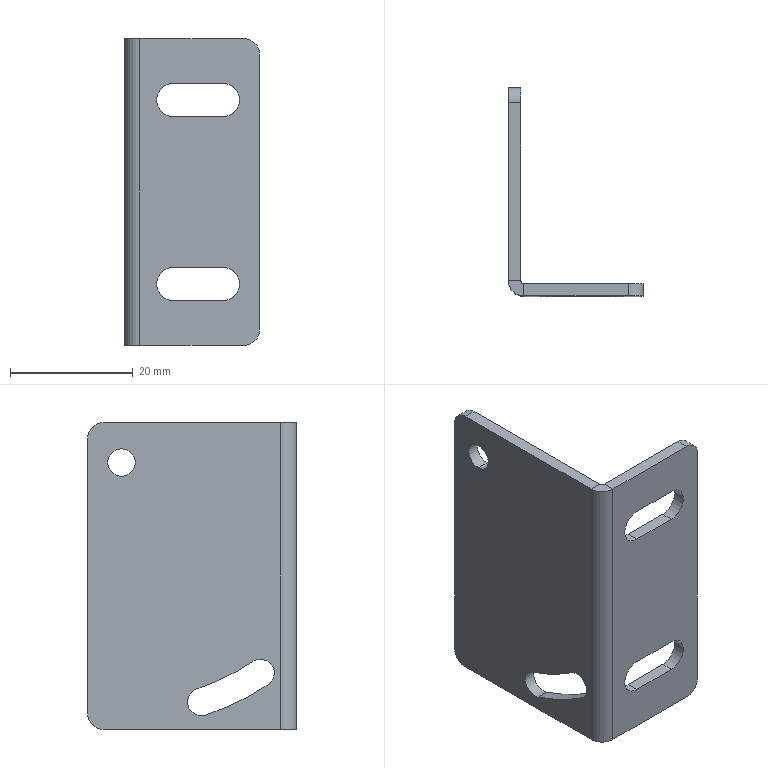Part | STEP file | KF-2212-060-004 | 1 solid | 33 faces | box 22 x 34 x 50 mm | volume 4893 mm3 | cylinder 17 | plane 16 | commonest cylinder face diameters 4.5 x5 5 x5 5.5 x4 1 x1 77.792 x1 86.792 x1
STEP:
#1=CARTESIAN_POINT('',(0.,26.5,45.75));
#2=VERTEX_POINT('',#1);
#3=CARTESIAN_POINT('',(0.,26.5,41.25));
#4=VERTEX_POINT('',#3);
#5=CARTESIAN_POINT('',(0.,26.5,43.5));
#6=DIRECTION('',(1.,0.,0.));
#7=DIRECTION('',(0.,0.,-1.));
#8=AXIS2_PLACEMENT_3D('',#5,#6,#7);
#9=CIRCLE('',#8,2.25);
#10=EDGE_CURVE('',#2,#4,#9,.T.);
#11=ORIENTED_EDGE('',*,*,#10,.T.);
#12=CARTESIAN_POINT('',(-2.,26.5,41.25));
#13=VERTEX_POINT('',#12);
#14=CARTESIAN_POINT('',(8.,26.5,41.25));
#15=DIRECTION('',(-1.,0.,0.));
#16=VECTOR('',#15,1000.);
#17=LINE('',#14,#16);
#18=EDGE_CURVE('',#4,#13,#17,.T.);
#19=ORIENTED_EDGE('',*,*,#18,.T.);
#20=CARTESIAN_POINT('',(-2.,26.5,45.75));
#21=VERTEX_POINT('',#20);
#22=CARTESIAN_POINT('',(-2.,26.5,43.5));
#23=DIRECTION('',(-1.,0.,0.));
#24=DIRECTION('',(0.,0.,1.));
#25=AXIS2_PLACEMENT_3D('',#22,#23,#24);
#26=CIRCLE('',#25,2.25);
#27=EDGE_CURVE('',#13,#21,#26,.T.);
#28=ORIENTED_EDGE('',*,*,#27,.T.);
#29=CARTESIAN_POINT('',(8.,26.5,45.75));
#30=DIRECTION('',(-1.,0.,0.));
#31=VECTOR('',#30,1000.);
#32=LINE('',#29,#31);
#33=EDGE_CURVE('',#2,#21,#32,.T.);
#34=ORIENTED_EDGE('',*,*,#33,.F.);
#35=EDGE_LOOP('',(#11,#19,#28,#34));
#36=FACE_OUTER_BOUND('',#35,.T.);
#37=CARTESIAN_POINT('',(8.,26.5,43.5));
#38=DIRECTION('',(-1.,0.,0.));
#39=DIRECTION('',(0.,0.,1.));
#40=AXIS2_PLACEMENT_3D('',#37,#38,#39);
#41=CYLINDRICAL_SURFACE('',#40,2.25);
#42=ADVANCED_FACE('',(#36),#41,.F.);
#43=CARTESIAN_POINT('',(0.,5.064,11.044));
#44=VERTEX_POINT('',#43);
#45=CARTESIAN_POINT('',(0.,3.825,11.416));
#46=VERTEX_POINT('',#45);
#47=CARTESIAN_POINT('',(0.,3.825,9.166));
#48=DIRECTION('',(1.,0.,0.));
#49=DIRECTION('',(0.,0.,-1.));
#50=AXIS2_PLACEMENT_3D('',#47,#48,#49);
#51=CIRCLE('',#50,2.25);
#52=EDGE_CURVE('',#44,#46,#51,.T.);
#53=ORIENTED_EDGE('',*,*,#52,.T.);
#54=CARTESIAN_POINT('',(-2.,3.825,11.416));
#55=VERTEX_POINT('',#54);
#56=CARTESIAN_POINT('',(8.,3.825,11.416));
#57=DIRECTION('',(-1.,0.,0.));
#58=VECTOR('',#57,1000.);
#59=LINE('',#56,#58);
#60=EDGE_CURVE('',#46,#55,#59,.T.);
#61=ORIENTED_EDGE('',*,*,#60,.T.);
#62=CARTESIAN_POINT('',(-2.,5.064,11.044));
#63=VERTEX_POINT('',#62);
#64=CARTESIAN_POINT('',(-2.,3.825,9.166));
#65=DIRECTION('',(-1.,0.,0.));
#66=DIRECTION('',(0.,0.,1.));
#67=AXIS2_PLACEMENT_3D('',#64,#65,#66);
#68=CIRCLE('',#67,2.25);
#69=EDGE_CURVE('',#55,#63,#68,.T.);
#70=ORIENTED_EDGE('',*,*,#69,.T.);
#71=CARTESIAN_POINT('',(8.,5.064,11.044));
#72=DIRECTION('',(-1.,0.,0.));
#73=VECTOR('',#72,1000.);
#74=LINE('',#71,#73);
#75=EDGE_CURVE('',#44,#63,#74,.T.);
#76=ORIENTED_EDGE('',*,*,#75,.F.);
#77=EDGE_LOOP('',(#53,#61,#70,#76));
#78=FACE_OUTER_BOUND('',#77,.T.);
#79=CARTESIAN_POINT('',(8.,3.825,9.166));
#80=DIRECTION('',(-1.,0.,0.));
#81=DIRECTION('',(0.,0.,1.));
#82=AXIS2_PLACEMENT_3D('',#79,#80,#81);
#83=CYLINDRICAL_SURFACE('',#82,2.25);
#84=ADVANCED_FACE('',(#78),#83,.F.);
#85=CARTESIAN_POINT('',(0.5,0.,50.));
#86=VERTEX_POINT('',#85);
#87=CARTESIAN_POINT('',(0.5,-2.,50.));
#88=VERTEX_POINT('',#87);
#89=CARTESIAN_POINT('',(0.5,0.,50.));
#90=DIRECTION('',(0.,-1.,0.));
#91=VECTOR('',#90,1000.);
#92=LINE('',#89,#91);
#93=EDGE_CURVE('',#86,#88,#92,.T.);
#94=ORIENTED_EDGE('',*,*,#93,.F.);
#95=CARTESIAN_POINT('',(0.,0.5,50.));
#96=VERTEX_POINT('',#95);
#97=CARTESIAN_POINT('',(0.5,0.5,50.));
#98=DIRECTION('',(0.,0.,1.));
#99=DIRECTION('',(-1.,0.,0.));
#100=AXIS2_PLACEMENT_3D('',#97,#98,#99);
#101=CIRCLE('',#100,0.5);
#102=EDGE_CURVE('',#96,#86,#101,.T.);
#103=ORIENTED_EDGE('',*,*,#102,.F.);
#104=CARTESIAN_POINT('',(-2.,0.5,50.));
#105=VERTEX_POINT('',#104);
#106=CARTESIAN_POINT('',(-2.,0.5,50.));
#107=DIRECTION('',(1.,0.,0.));
#108=VECTOR('',#107,1000.);
#109=LINE('',#106,#108);
#110=EDGE_CURVE('',#105,#96,#109,.T.);
#111=ORIENTED_EDGE('',*,*,#110,.F.);
#112=CARTESIAN_POINT('',(0.5,0.5,50.));
#113=DIRECTION('',(0.,0.,1.));
#114=DIRECTION('',(1.,0.,0.));
#115=AXIS2_PLACEMENT_3D('',#112,#113,#114);
#116=CIRCLE('',#115,2.5);
#117=EDGE_CURVE('',#105,#88,#116,.T.);
#118=ORIENTED_EDGE('',*,*,#117,.T.);
#119=EDGE_LOOP('',(#94,#103,#111,#118));
#120=FACE_OUTER_BOUND('',#119,.T.);
#121=CARTESIAN_POINT('',(0.5,0.,50.));
#122=DIRECTION('',(0.,0.,1.));
#123=DIRECTION('',(1.,0.,0.));
#124=AXIS2_PLACEMENT_3D('',#121,#122,#123);
#125=PLANE('',#124);
#126=ADVANCED_FACE('',(#120),#125,.T.);
#127=CARTESIAN_POINT('',(17.5,-2.,50.));
#128=VERTEX_POINT('',#127);
#129=CARTESIAN_POINT('',(0.,-2.,50.));
#130=DIRECTION('',(1.,0.,0.));
#131=VECTOR('',#130,1000.);
#132=LINE('',#129,#131);
#133=EDGE_CURVE('',#88,#128,#132,.T.);
#134=ORIENTED_EDGE('',*,*,#133,.T.);
#135=CARTESIAN_POINT('',(17.5,0.,50.));
#136=VERTEX_POINT('',#135);
#137=CARTESIAN_POINT('',(17.5,0.5,50.));
#138=DIRECTION('',(0.,1.,0.));
#139=VECTOR('',#138,1000.);
#140=LINE('',#137,#139);
#141=EDGE_CURVE('',#128,#136,#140,.T.);
#142=ORIENTED_EDGE('',*,*,#141,.T.);
#143=CARTESIAN_POINT('',(0.,0.,50.));
#144=DIRECTION('',(1.,0.,0.));
#145=VECTOR('',#144,1000.);
#146=LINE('',#143,#145);
#147=EDGE_CURVE('',#86,#136,#146,.T.);
#148=ORIENTED_EDGE('',*,*,#147,.F.);
#149=ORIENTED_EDGE('',*,*,#93,.T.);
#150=EDGE_LOOP('',(#134,#142,#148,#149));
#151=FACE_OUTER_BOUND('',#150,.T.);
#152=CARTESIAN_POINT('',(-2.,0.5,50.));
#153=DIRECTION('',(0.,0.,1.));
#154=DIRECTION('',(1.,0.,0.));
#155=AXIS2_PLACEMENT_3D('',#152,#153,#154);
#156=PLANE('',#155);
#157=ADVANCED_FACE('',(#151),#156,.T.);
#158=CARTESIAN_POINT('',(0.,0.5,0.));
#159=VERTEX_POINT('',#158);
#160=CARTESIAN_POINT('',(-2.,0.5,0.));
#161=VERTEX_POINT('',#160);
#162=CARTESIAN_POINT('',(0.,0.5,0.));
#163=DIRECTION('',(-1.,0.,0.));
#164=VECTOR('',#163,1000.);
#165=LINE('',#162,#164);
#166=EDGE_CURVE('',#159,#161,#165,.T.);
#167=ORIENTED_EDGE('',*,*,#166,.F.);
#168=CARTESIAN_POINT('',(0.5,0.,0.));
#169=VERTEX_POINT('',#168);
#170=CARTESIAN_POINT('',(0.5,0.5,0.));
#171=DIRECTION('',(0.,0.,1.));
#172=DIRECTION('',(-1.,0.,0.));
#173=AXIS2_PLACEMENT_3D('',#170,#171,#172);
#174=CIRCLE('',#173,0.5);
#175=EDGE_CURVE('',#159,#169,#174,.T.);
#176=ORIENTED_EDGE('',*,*,#175,.T.);
#177=CARTESIAN_POINT('',(0.5,-2.,0.));
#178=VERTEX_POINT('',#177);
#179=CARTESIAN_POINT('',(0.5,-2.,0.));
#180=DIRECTION('',(0.,1.,0.));
#181=VECTOR('',#180,1000.);
#182=LINE('',#179,#181);
#183=EDGE_CURVE('',#178,#169,#182,.T.);
#184=ORIENTED_EDGE('',*,*,#183,.F.);
#185=CARTESIAN_POINT('',(0.5,0.5,0.));
#186=DIRECTION('',(0.,0.,1.));
#187=DIRECTION('',(1.,0.,0.));
#188=AXIS2_PLACEMENT_3D('',#185,#186,#187);
#189=CIRCLE('',#188,2.5);
#190=EDGE_CURVE('',#161,#178,#189,.T.);
#191=ORIENTED_EDGE('',*,*,#190,.F.);
#192=EDGE_LOOP('',(#167,#176,#184,#191));
#193=FACE_OUTER_BOUND('',#192,.T.);
#194=CARTESIAN_POINT('',(0.,0.5,0.));
#195=DIRECTION('',(0.,0.,-1.));
#196=DIRECTION('',(-1.,0.,0.));
#197=AXIS2_PLACEMENT_3D('',#194,#195,#196);
#198=PLANE('',#197);
#199=ADVANCED_FACE('',(#193),#198,.T.);
#200=CARTESIAN_POINT('',(-2.,29.5,0.));
#201=VERTEX_POINT('',#200);
#202=CARTESIAN_POINT('',(-2.,0.,0.));
#203=DIRECTION('',(0.,-1.,0.));
#204=VECTOR('',#203,1000.);
#205=LINE('',#202,#204);
#206=EDGE_CURVE('',#201,#161,#205,.T.);
#207=ORIENTED_EDGE('',*,*,#206,.F.);
#208=CARTESIAN_POINT('',(0.,29.5,0.));
#209=VERTEX_POINT('',#208);
#210=CARTESIAN_POINT('',(0.5,29.5,0.));
#211=DIRECTION('',(1.,0.,0.));
#212=VECTOR('',#211,1000.);
#213=LINE('',#210,#212);
#214=EDGE_CURVE('',#201,#209,#213,.T.);
#215=ORIENTED_EDGE('',*,*,#214,.T.);
#216=CARTESIAN_POINT('',(0.,0.,0.));
#217=DIRECTION('',(0.,-1.,0.));
#218=VECTOR('',#217,1000.);
#219=LINE('',#216,#218);
#220=EDGE_CURVE('',#209,#159,#219,.T.);
#221=ORIENTED_EDGE('',*,*,#220,.T.);
#222=ORIENTED_EDGE('',*,*,#166,.T.);
#223=EDGE_LOOP('',(#207,#215,#221,#222));
#224=FACE_OUTER_BOUND('',#223,.T.);
#225=CARTESIAN_POINT('',(0.5,-2.,0.));
#226=DIRECTION('',(0.,0.,-1.));
#227=DIRECTION('',(-1.,0.,0.));
#228=AXIS2_PLACEMENT_3D('',#225,#226,#227);
#229=PLANE('',#228);
#230=ADVANCED_FACE('',(#224),#229,.T.);
#231=CARTESIAN_POINT('',(6.,-2.,7.25));
#232=VERTEX_POINT('',#231);
#233=CARTESIAN_POINT('',(14.,-2.,7.25));
#234=VERTEX_POINT('',#233);
#235=CARTESIAN_POINT('',(6.,-2.,7.25));
#236=DIRECTION('',(1.,0.,0.));
#237=VECTOR('',#236,1000.);
#238=LINE('',#235,#237);
#239=EDGE_CURVE('',#232,#234,#238,.T.);
#240=ORIENTED_EDGE('',*,*,#239,.F.);
#241=CARTESIAN_POINT('',(6.,-2.,12.75));
#242=VERTEX_POINT('',#241);
#243=CARTESIAN_POINT('',(6.,-2.,10.));
#244=DIRECTION('',(0.,-1.,0.));
#245=DIRECTION('',(0.,0.,-1.));
#246=AXIS2_PLACEMENT_3D('',#243,#244,#245);
#247=CIRCLE('',#246,2.75);
#248=EDGE_CURVE('',#242,#232,#247,.T.);
#249=ORIENTED_EDGE('',*,*,#248,.F.);
#250=CARTESIAN_POINT('',(14.,-2.,12.75));
#251=VERTEX_POINT('',#250);
#252=CARTESIAN_POINT('',(6.,-2.,12.75));
#253=DIRECTION('',(-1.,0.,0.));
#254=VECTOR('',#253,1000.);
#255=LINE('',#252,#254);
#256=EDGE_CURVE('',#251,#242,#255,.T.);
#257=ORIENTED_EDGE('',*,*,#256,.F.);
#258=CARTESIAN_POINT('',(14.,-2.,10.));
#259=DIRECTION('',(0.,-1.,0.));
#260=DIRECTION('',(0.,0.,-1.));
#261=AXIS2_PLACEMENT_3D('',#258,#259,#260);
#262=CIRCLE('',#261,2.75);
#263=EDGE_CURVE('',#234,#251,#262,.T.);
#264=ORIENTED_EDGE('',*,*,#263,.F.);
#265=EDGE_LOOP('',(#240,#249,#257,#264));
#266=FACE_BOUND('',#265,.T.);
#267=CARTESIAN_POINT('',(6.,-2.,37.25));
#268=VERTEX_POINT('',#267);
#269=CARTESIAN_POINT('',(14.,-2.,37.25));
#270=VERTEX_POINT('',#269);
#271=CARTESIAN_POINT('',(6.,-2.,37.25));
#272=DIRECTION('',(1.,0.,0.));
#273=VECTOR('',#272,1000.);
#274=LINE('',#271,#273);
#275=EDGE_CURVE('',#268,#270,#274,.T.);
#276=ORIENTED_EDGE('',*,*,#275,.F.);
#277=CARTESIAN_POINT('',(6.,-2.,42.75));
#278=VERTEX_POINT('',#277);
#279=CARTESIAN_POINT('',(6.,-2.,40.));
#280=DIRECTION('',(0.,-1.,0.));
#281=DIRECTION('',(0.,0.,-1.));
#282=AXIS2_PLACEMENT_3D('',#279,#280,#281);
#283=CIRCLE('',#282,2.75);
#284=EDGE_CURVE('',#278,#268,#283,.T.);
#285=ORIENTED_EDGE('',*,*,#284,.F.);
#286=CARTESIAN_POINT('',(14.,-2.,42.75));
#287=VERTEX_POINT('',#286);
#288=CARTESIAN_POINT('',(6.,-2.,42.75));
#289=DIRECTION('',(-1.,0.,0.));
#290=VECTOR('',#289,1000.);
#291=LINE('',#288,#290);
#292=EDGE_CURVE('',#287,#278,#291,.T.);
#293=ORIENTED_EDGE('',*,*,#292,.F.);
#294=CARTESIAN_POINT('',(14.,-2.,40.));
#295=DIRECTION('',(0.,-1.,0.));
#296=DIRECTION('',(0.,0.,-1.));
#297=AXIS2_PLACEMENT_3D('',#294,#295,#296);
#298=CIRCLE('',#297,2.75);
#299=EDGE_CURVE('',#270,#287,#298,.T.);
#300=ORIENTED_EDGE('',*,*,#299,.F.);
#301=EDGE_LOOP('',(#276,#285,#293,#300));
#302=FACE_BOUND('',#301,.T.);
#303=CARTESIAN_POINT('',(17.5,-2.,0.));
#304=VERTEX_POINT('',#303);
#305=CARTESIAN_POINT('',(0.,-2.,0.));
#306=DIRECTION('',(1.,0.,0.));
#307=VECTOR('',#306,1000.);
#308=LINE('',#305,#307);
#309=EDGE_CURVE('',#178,#304,#308,.T.);
#310=ORIENTED_EDGE('',*,*,#309,.T.);
#311=CARTESIAN_POINT('',(20.,-2.,2.5));
#312=VERTEX_POINT('',#311);
#313=CARTESIAN_POINT('',(17.5,-2.,2.5));
#314=DIRECTION('',(0.,-1.,0.));
#315=DIRECTION('',(0.,0.,1.));
#316=AXIS2_PLACEMENT_3D('',#313,#314,#315);
#317=CIRCLE('',#316,2.5);
#318=EDGE_CURVE('',#304,#312,#317,.T.);
#319=ORIENTED_EDGE('',*,*,#318,.T.);
#320=CARTESIAN_POINT('',(20.,-2.,47.5));
#321=VERTEX_POINT('',#320);
#322=CARTESIAN_POINT('',(20.,-2.,50.));
#323=DIRECTION('',(0.,0.,-1.));
#324=VECTOR('',#323,1000.);
#325=LINE('',#322,#324);
#326=EDGE_CURVE('',#321,#312,#325,.T.);
#327=ORIENTED_EDGE('',*,*,#326,.F.);
#328=CARTESIAN_POINT('',(17.5,-2.,47.5));
#329=DIRECTION('',(0.,-1.,0.));
#330=DIRECTION('',(0.,0.,1.));
#331=AXIS2_PLACEMENT_3D('',#328,#329,#330);
#332=CIRCLE('',#331,2.5);
#333=EDGE_CURVE('',#321,#128,#332,.T.);
#334=ORIENTED_EDGE('',*,*,#333,.T.);
#335=ORIENTED_EDGE('',*,*,#133,.F.);
#336=CARTESIAN_POINT('',(0.5,-2.,50.));
#337=DIRECTION('',(0.,0.,-1.));
#338=VECTOR('',#337,1000.);
#339=LINE('',#336,#338);
#340=EDGE_CURVE('',#88,#178,#339,.T.);
#341=ORIENTED_EDGE('',*,*,#340,.T.);
#342=EDGE_LOOP('',(#310,#319,#327,#334,#335,#341));
#343=FACE_OUTER_BOUND('',#342,.T.);
#344=CARTESIAN_POINT('',(0.,-2.,50.));
#345=DIRECTION('',(0.,1.,0.));
#346=DIRECTION('',(0.,0.,1.));
#347=AXIS2_PLACEMENT_3D('',#344,#345,#346);
#348=PLANE('',#347);
#349=ADVANCED_FACE('',(#266,#302,#343),#348,.F.);
#350=ORIENTED_EDGE('',*,*,#326,.T.);
#351=CARTESIAN_POINT('',(20.,0.,2.5));
#352=VERTEX_POINT('',#351);
#353=CARTESIAN_POINT('',(20.,0.,2.5));
#354=DIRECTION('',(0.,1.,0.));
#355=VECTOR('',#354,1000.);
#356=LINE('',#353,#355);
#357=EDGE_CURVE('',#312,#352,#356,.T.);
#358=ORIENTED_EDGE('',*,*,#357,.T.);
#359=CARTESIAN_POINT('',(20.,0.,47.5));
#360=VERTEX_POINT('',#359);
#361=CARTESIAN_POINT('',(20.,0.,50.));
#362=DIRECTION('',(0.,0.,-1.));
#363=VECTOR('',#362,1000.);
#364=LINE('',#361,#363);
#365=EDGE_CURVE('',#360,#352,#364,.T.);
#366=ORIENTED_EDGE('',*,*,#365,.F.);
#367=CARTESIAN_POINT('',(20.,0.,47.5));
#368=DIRECTION('',(0.,-1.,0.));
#369=VECTOR('',#368,1000.);
#370=LINE('',#367,#369);
#371=EDGE_CURVE('',#360,#321,#370,.T.);
#372=ORIENTED_EDGE('',*,*,#371,.T.);
#373=EDGE_LOOP('',(#350,#358,#366,#372));
#374=FACE_OUTER_BOUND('',#373,.T.);
#375=CARTESIAN_POINT('',(20.,0.,50.));
#376=DIRECTION('',(1.,0.,0.));
#377=DIRECTION('',(0.,0.,-1.));
#378=AXIS2_PLACEMENT_3D('',#375,#376,#377);
#379=PLANE('',#378);
#380=ADVANCED_FACE('',(#374),#379,.T.);
#381=CARTESIAN_POINT('',(6.,0.,7.25));
#382=VERTEX_POINT('',#381);
#383=CARTESIAN_POINT('',(6.,0.,12.75));
#384=VERTEX_POINT('',#383);
#385=CARTESIAN_POINT('',(6.,0.,10.));
#386=DIRECTION('',(0.,1.,0.));
#387=DIRECTION('',(0.,0.,1.));
#388=AXIS2_PLACEMENT_3D('',#385,#386,#387);
#389=CIRCLE('',#388,2.75);
#390=EDGE_CURVE('',#382,#384,#389,.T.);
#391=ORIENTED_EDGE('',*,*,#390,.F.);
#392=CARTESIAN_POINT('',(14.,0.,7.25));
#393=VERTEX_POINT('',#392);
#394=CARTESIAN_POINT('',(0.,0.,7.25));
#395=DIRECTION('',(-1.,0.,0.));
#396=VECTOR('',#395,1000.);
#397=LINE('',#394,#396);
#398=EDGE_CURVE('',#393,#382,#397,.T.);
#399=ORIENTED_EDGE('',*,*,#398,.F.);
#400=CARTESIAN_POINT('',(14.,0.,12.75));
#401=VERTEX_POINT('',#400);
#402=CARTESIAN_POINT('',(14.,0.,10.));
#403=DIRECTION('',(0.,1.,0.));
#404=DIRECTION('',(0.,0.,1.));
#405=AXIS2_PLACEMENT_3D('',#402,#403,#404);
#406=CIRCLE('',#405,2.75);
#407=EDGE_CURVE('',#401,#393,#406,.T.);
#408=ORIENTED_EDGE('',*,*,#407,.F.);
#409=CARTESIAN_POINT('',(0.,0.,12.75));
#410=DIRECTION('',(1.,0.,0.));
#411=VECTOR('',#410,1000.);
#412=LINE('',#409,#411);
#413=EDGE_CURVE('',#384,#401,#412,.T.);
#414=ORIENTED_EDGE('',*,*,#413,.F.);
#415=EDGE_LOOP('',(#391,#399,#408,#414));
#416=FACE_BOUND('',#415,.T.);
#417=CARTESIAN_POINT('',(6.,0.,37.25));
#418=VERTEX_POINT('',#417);
#419=CARTESIAN_POINT('',(6.,0.,42.75));
#420=VERTEX_POINT('',#419);
#421=CARTESIAN_POINT('',(6.,0.,40.));
#422=DIRECTION('',(0.,1.,0.));
#423=DIRECTION('',(0.,0.,1.));
#424=AXIS2_PLACEMENT_3D('',#421,#422,#423);
#425=CIRCLE('',#424,2.75);
#426=EDGE_CURVE('',#418,#420,#425,.T.);
#427=ORIENTED_EDGE('',*,*,#426,.F.);
#428=CARTESIAN_POINT('',(14.,0.,37.25));
#429=VERTEX_POINT('',#428);
#430=CARTESIAN_POINT('',(0.,0.,37.25));
#431=DIRECTION('',(-1.,0.,0.));
#432=VECTOR('',#431,1000.);
#433=LINE('',#430,#432);
#434=EDGE_CURVE('',#429,#418,#433,.T.);
#435=ORIENTED_EDGE('',*,*,#434,.F.);
#436=CARTESIAN_POINT('',(14.,0.,42.75));
#437=VERTEX_POINT('',#436);
#438=CARTESIAN_POINT('',(14.,0.,40.));
#439=DIRECTION('',(0.,1.,0.));
#440=DIRECTION('',(0.,0.,1.));
#441=AXIS2_PLACEMENT_3D('',#438,#439,#440);
#442=CIRCLE('',#441,2.75);
#443=EDGE_CURVE('',#437,#429,#442,.T.);
#444=ORIENTED_EDGE('',*,*,#443,.F.);
#445=CARTESIAN_POINT('',(0.,0.,42.75));
#446=DIRECTION('',(1.,0.,0.));
#447=VECTOR('',#446,1000.);
#448=LINE('',#445,#447);
#449=EDGE_CURVE('',#420,#437,#448,.T.);
#450=ORIENTED_EDGE('',*,*,#449,.F.);
#451=EDGE_LOOP('',(#427,#435,#444,#450));
#452=FACE_BOUND('',#451,.T.);
#453=ORIENTED_EDGE('',*,*,#365,.T.);
#454=CARTESIAN_POINT('',(17.5,0.,0.));
#455=VERTEX_POINT('',#454);
#456=CARTESIAN_POINT('',(17.5,0.,2.5));
#457=DIRECTION('',(0.,1.,0.));
#458=DIRECTION('',(0.,0.,1.));
#459=AXIS2_PLACEMENT_3D('',#456,#457,#458);
#460=CIRCLE('',#459,2.5);
#461=EDGE_CURVE('',#352,#455,#460,.T.);
#462=ORIENTED_EDGE('',*,*,#461,.T.);
#463=CARTESIAN_POINT('',(0.,0.,0.));
#464=DIRECTION('',(1.,0.,0.));
#465=VECTOR('',#464,1000.);
#466=LINE('',#463,#465);
#467=EDGE_CURVE('',#169,#455,#466,.T.);
#468=ORIENTED_EDGE('',*,*,#467,.F.);
#469=CARTESIAN_POINT('',(0.5,0.,50.));
#470=DIRECTION('',(0.,0.,-1.));
#471=VECTOR('',#470,1000.);
#472=LINE('',#469,#471);
#473=EDGE_CURVE('',#86,#169,#472,.T.);
#474=ORIENTED_EDGE('',*,*,#473,.F.);
#475=ORIENTED_EDGE('',*,*,#147,.T.);
#476=CARTESIAN_POINT('',(17.5,0.,47.5));
#477=DIRECTION('',(0.,1.,0.));
#478=DIRECTION('',(0.,0.,1.));
#479=AXIS2_PLACEMENT_3D('',#476,#477,#478);
#480=CIRCLE('',#479,2.5);
#481=EDGE_CURVE('',#136,#360,#480,.T.);
#482=ORIENTED_EDGE('',*,*,#481,.T.);
#483=EDGE_LOOP('',(#453,#462,#468,#474,#475,#482));
#484=FACE_OUTER_BOUND('',#483,.T.);
#485=CARTESIAN_POINT('',(0.,0.,50.));
#486=DIRECTION('',(0.,1.,0.));
#487=DIRECTION('',(0.,0.,1.));
#488=AXIS2_PLACEMENT_3D('',#485,#486,#487);
#489=PLANE('',#488);
#490=ADVANCED_FACE('',(#416,#452,#484),#489,.T.);
#491=ORIENTED_EDGE('',*,*,#175,.F.);
#492=CARTESIAN_POINT('',(0.,0.5,50.));
#493=DIRECTION('',(0.,0.,-1.));
#494=VECTOR('',#493,1000.);
#495=LINE('',#492,#494);
#496=EDGE_CURVE('',#96,#159,#495,.T.);
#497=ORIENTED_EDGE('',*,*,#496,.F.);
#498=ORIENTED_EDGE('',*,*,#102,.T.);
#499=ORIENTED_EDGE('',*,*,#473,.T.);
#500=EDGE_LOOP('',(#491,#497,#498,#499));
#501=FACE_OUTER_BOUND('',#500,.T.);
#502=CARTESIAN_POINT('',(0.5,0.5,50.));
#503=DIRECTION('',(0.,0.,-1.));
#504=DIRECTION('',(-1.,0.,0.));
#505=AXIS2_PLACEMENT_3D('',#502,#503,#504);
#506=CYLINDRICAL_SURFACE('',#505,0.5);
#507=ADVANCED_FACE('',(#501),#506,.F.);
#508=ORIENTED_EDGE('',*,*,#10,.F.);
#509=CARTESIAN_POINT('',(0.,26.5,43.5));
#510=DIRECTION('',(1.,0.,0.));
#511=DIRECTION('',(0.,0.,-1.));
#512=AXIS2_PLACEMENT_3D('',#509,#510,#511);
#513=CIRCLE('',#512,2.25);
#514=EDGE_CURVE('',#4,#2,#513,.T.);
#515=ORIENTED_EDGE('',*,*,#514,.F.);
#516=EDGE_LOOP('',(#508,#515));
#517=FACE_BOUND('',#516,.T.);
#518=CARTESIAN_POINT('',(0.,12.772,2.333));
#519=VERTEX_POINT('',#518);
#520=CARTESIAN_POINT('',(0.,14.195,6.602));
#521=VERTEX_POINT('',#520);
#522=CARTESIAN_POINT('',(0.,13.483,4.467));
#523=DIRECTION('',(1.,0.,0.));
#524=DIRECTION('',(0.,0.,-1.));
#525=AXIS2_PLACEMENT_3D('',#522,#523,#524);
#526=CIRCLE('',#525,2.25);
#527=EDGE_CURVE('',#519,#521,#526,.T.);
#528=ORIENTED_EDGE('',*,*,#527,.F.);
#529=CARTESIAN_POINT('',(0.,2.585,7.289));
#530=VERTEX_POINT('',#529);
#531=CARTESIAN_POINT('',(0.,26.5,43.5));
#532=DIRECTION('',(1.,0.,0.));
#533=DIRECTION('',(0.,0.,-1.));
#534=AXIS2_PLACEMENT_3D('',#531,#532,#533);
#535=CIRCLE('',#534,43.396);
#536=EDGE_CURVE('',#530,#519,#535,.T.);
#537=ORIENTED_EDGE('',*,*,#536,.F.);
#538=CARTESIAN_POINT('',(0.,3.825,9.166));
#539=DIRECTION('',(1.,0.,0.));
#540=DIRECTION('',(0.,0.,-1.));
#541=AXIS2_PLACEMENT_3D('',#538,#539,#540);
#542=CIRCLE('',#541,2.25);
#543=EDGE_CURVE('',#46,#530,#542,.T.);
#544=ORIENTED_EDGE('',*,*,#543,.F.);
#545=ORIENTED_EDGE('',*,*,#52,.F.);
#546=CARTESIAN_POINT('',(0.,26.5,43.5));
#547=DIRECTION('',(-1.,0.,0.));
#548=DIRECTION('',(0.,0.,-1.));
#549=AXIS2_PLACEMENT_3D('',#546,#547,#548);
#550=CIRCLE('',#549,38.896);
#551=EDGE_CURVE('',#521,#44,#550,.T.);
#552=ORIENTED_EDGE('',*,*,#551,.F.);
#553=EDGE_LOOP('',(#528,#537,#544,#545,#552));
#554=FACE_BOUND('',#553,.T.);
#555=CARTESIAN_POINT('',(0.,32.,47.5));
#556=VERTEX_POINT('',#555);
#557=CARTESIAN_POINT('',(0.,32.,2.5));
#558=VERTEX_POINT('',#557);
#559=CARTESIAN_POINT('',(0.,32.,50.));
#560=DIRECTION('',(0.,0.,-1.));
#561=VECTOR('',#560,1000.);
#562=LINE('',#559,#561);
#563=EDGE_CURVE('',#556,#558,#562,.T.);
#564=ORIENTED_EDGE('',*,*,#563,.F.);
#565=CARTESIAN_POINT('',(0.,29.5,50.));
#566=VERTEX_POINT('',#565);
#567=CARTESIAN_POINT('',(0.,29.5,47.5));
#568=DIRECTION('',(1.,0.,0.));
#569=DIRECTION('',(0.,0.,-1.));
#570=AXIS2_PLACEMENT_3D('',#567,#568,#569);
#571=CIRCLE('',#570,2.5);
#572=EDGE_CURVE('',#556,#566,#571,.T.);
#573=ORIENTED_EDGE('',*,*,#572,.T.);
#574=CARTESIAN_POINT('',(0.,0.,50.));
#575=DIRECTION('',(0.,-1.,0.));
#576=VECTOR('',#575,1000.);
#577=LINE('',#574,#576);
#578=EDGE_CURVE('',#566,#96,#577,.T.);
#579=ORIENTED_EDGE('',*,*,#578,.T.);
#580=ORIENTED_EDGE('',*,*,#496,.T.);
#581=ORIENTED_EDGE('',*,*,#220,.F.);
#582=CARTESIAN_POINT('',(0.,29.5,2.5));
#583=DIRECTION('',(1.,0.,0.));
#584=DIRECTION('',(0.,0.,-1.));
#585=AXIS2_PLACEMENT_3D('',#582,#583,#584);
#586=CIRCLE('',#585,2.5);
#587=EDGE_CURVE('',#209,#558,#586,.T.);
#588=ORIENTED_EDGE('',*,*,#587,.T.);
#589=EDGE_LOOP('',(#564,#573,#579,#580,#581,#588));
#590=FACE_OUTER_BOUND('',#589,.T.);
#591=CARTESIAN_POINT('',(0.,0.,50.));
#592=DIRECTION('',(1.,0.,0.));
#593=DIRECTION('',(0.,0.,-1.));
#594=AXIS2_PLACEMENT_3D('',#591,#592,#593);
#595=PLANE('',#594);
#596=ADVANCED_FACE('',(#517,#554,#590),#595,.T.);
#597=CARTESIAN_POINT('',(-2.,32.,47.5));
#598=VERTEX_POINT('',#597);
#599=CARTESIAN_POINT('',(-2.,32.,2.5));
#600=VERTEX_POINT('',#599);
#601=CARTESIAN_POINT('',(-2.,32.,50.));
#602=DIRECTION('',(0.,0.,-1.));
#603=VECTOR('',#602,1000.);
#604=LINE('',#601,#603);
#605=EDGE_CURVE('',#598,#600,#604,.T.);
#606=ORIENTED_EDGE('',*,*,#605,.F.);
#607=CARTESIAN_POINT('',(0.,32.,47.5));
#608=DIRECTION('',(1.,0.,0.));
#609=VECTOR('',#608,1000.);
#610=LINE('',#607,#609);
#611=EDGE_CURVE('',#598,#556,#610,.T.);
#612=ORIENTED_EDGE('',*,*,#611,.T.);
#613=ORIENTED_EDGE('',*,*,#563,.T.);
#614=CARTESIAN_POINT('',(-2.,32.,2.5));
#615=DIRECTION('',(-1.,0.,0.));
#616=VECTOR('',#615,1000.);
#617=LINE('',#614,#616);
#618=EDGE_CURVE('',#558,#600,#617,.T.);
#619=ORIENTED_EDGE('',*,*,#618,.T.);
#620=EDGE_LOOP('',(#606,#612,#613,#619));
#621=FACE_OUTER_BOUND('',#620,.T.);
#622=CARTESIAN_POINT('',(-2.,32.,50.));
#623=DIRECTION('',(0.,1.,0.));
#624=DIRECTION('',(0.,0.,1.));
#625=AXIS2_PLACEMENT_3D('',#622,#623,#624);
#626=PLANE('',#625);
#627=ADVANCED_FACE('',(#621),#626,.T.);
#628=CARTESIAN_POINT('',(-2.,26.5,43.5));
#629=DIRECTION('',(-1.,0.,0.));
#630=DIRECTION('',(0.,0.,1.));
#631=AXIS2_PLACEMENT_3D('',#628,#629,#630);
#632=CIRCLE('',#631,2.25);
#633=EDGE_CURVE('',#21,#13,#632,.T.);
#634=ORIENTED_EDGE('',*,*,#633,.F.);
#635=ORIENTED_EDGE('',*,*,#27,.F.);
#636=EDGE_LOOP('',(#634,#635));
#637=FACE_BOUND('',#636,.T.);
#638=CARTESIAN_POINT('',(-2.,12.772,2.333));
#639=VERTEX_POINT('',#638);
#640=CARTESIAN_POINT('',(-2.,2.585,7.289));
#641=VERTEX_POINT('',#640);
#642=CARTESIAN_POINT('',(-2.,26.5,43.5));
#643=DIRECTION('',(-1.,0.,0.));
#644=DIRECTION('',(0.,0.,1.));
#645=AXIS2_PLACEMENT_3D('',#642,#643,#644);
#646=CIRCLE('',#645,43.396);
#647=EDGE_CURVE('',#639,#641,#646,.T.);
#648=ORIENTED_EDGE('',*,*,#647,.F.);
#649=CARTESIAN_POINT('',(-2.,14.195,6.602));
#650=VERTEX_POINT('',#649);
#651=CARTESIAN_POINT('',(-2.,13.483,4.467));
#652=DIRECTION('',(-1.,0.,0.));
#653=DIRECTION('',(0.,0.,1.));
#654=AXIS2_PLACEMENT_3D('',#651,#652,#653);
#655=CIRCLE('',#654,2.25);
#656=EDGE_CURVE('',#650,#639,#655,.T.);
#657=ORIENTED_EDGE('',*,*,#656,.F.);
#658=CARTESIAN_POINT('',(-2.,26.5,43.5));
#659=DIRECTION('',(1.,0.,0.));
#660=DIRECTION('',(0.,0.,1.));
#661=AXIS2_PLACEMENT_3D('',#658,#659,#660);
#662=CIRCLE('',#661,38.896);
#663=EDGE_CURVE('',#63,#650,#662,.T.);
#664=ORIENTED_EDGE('',*,*,#663,.F.);
#665=ORIENTED_EDGE('',*,*,#69,.F.);
#666=CARTESIAN_POINT('',(-2.,3.825,9.166));
#667=DIRECTION('',(-1.,0.,0.));
#668=DIRECTION('',(0.,0.,1.));
#669=AXIS2_PLACEMENT_3D('',#666,#667,#668);
#670=CIRCLE('',#669,2.25);
#671=EDGE_CURVE('',#641,#55,#670,.T.);
#672=ORIENTED_EDGE('',*,*,#671,.F.);
#673=EDGE_LOOP('',(#648,#657,#664,#665,#672));
#674=FACE_BOUND('',#673,.T.);
#675=CARTESIAN_POINT('',(-2.,29.5,50.));
#676=VERTEX_POINT('',#675);
#677=CARTESIAN_POINT('',(-2.,0.,50.));
#678=DIRECTION('',(0.,-1.,0.));
#679=VECTOR('',#678,1000.);
#680=LINE('',#677,#679);
#681=EDGE_CURVE('',#676,#105,#680,.T.);
#682=ORIENTED_EDGE('',*,*,#681,.F.);
#683=CARTESIAN_POINT('',(-2.,29.5,47.5));
#684=DIRECTION('',(-1.,0.,0.));
#685=DIRECTION('',(0.,0.,-1.));
#686=AXIS2_PLACEMENT_3D('',#683,#684,#685);
#687=CIRCLE('',#686,2.5);
#688=EDGE_CURVE('',#676,#598,#687,.T.);
#689=ORIENTED_EDGE('',*,*,#688,.T.);
#690=ORIENTED_EDGE('',*,*,#605,.T.);
#691=CARTESIAN_POINT('',(-2.,29.5,2.5));
#692=DIRECTION('',(-1.,0.,0.));
#693=DIRECTION('',(0.,0.,-1.));
#694=AXIS2_PLACEMENT_3D('',#691,#692,#693);
#695=CIRCLE('',#694,2.5);
#696=EDGE_CURVE('',#600,#201,#695,.T.);
#697=ORIENTED_EDGE('',*,*,#696,.T.);
#698=ORIENTED_EDGE('',*,*,#206,.T.);
#699=CARTESIAN_POINT('',(-2.,0.5,50.));
#700=DIRECTION('',(0.,0.,-1.));
#701=VECTOR('',#700,1000.);
#702=LINE('',#699,#701);
#703=EDGE_CURVE('',#105,#161,#702,.T.);
#704=ORIENTED_EDGE('',*,*,#703,.F.);
#705=EDGE_LOOP('',(#682,#689,#690,#697,#698,#704));
#706=FACE_OUTER_BOUND('',#705,.T.);
#707=CARTESIAN_POINT('',(-2.,0.,50.));
#708=DIRECTION('',(1.,0.,0.));
#709=DIRECTION('',(0.,0.,-1.));
#710=AXIS2_PLACEMENT_3D('',#707,#708,#709);
#711=PLANE('',#710);
#712=ADVANCED_FACE('',(#637,#674,#706),#711,.F.);
#713=ORIENTED_EDGE('',*,*,#190,.T.);
#714=ORIENTED_EDGE('',*,*,#340,.F.);
#715=ORIENTED_EDGE('',*,*,#117,.F.);
#716=ORIENTED_EDGE('',*,*,#703,.T.);
#717=EDGE_LOOP('',(#713,#714,#715,#716));
#718=FACE_OUTER_BOUND('',#717,.T.);
#719=CARTESIAN_POINT('',(0.5,0.5,50.));
#720=DIRECTION('',(0.,0.,-1.));
#721=DIRECTION('',(-1.,0.,0.));
#722=AXIS2_PLACEMENT_3D('',#719,#720,#721);
#723=CYLINDRICAL_SURFACE('',#722,2.5);
#724=ADVANCED_FACE('',(#718),#723,.T.);
#725=ORIENTED_EDGE('',*,*,#578,.F.);
#726=CARTESIAN_POINT('',(-2.,29.5,50.));
#727=DIRECTION('',(-1.,0.,0.));
#728=VECTOR('',#727,1000.);
#729=LINE('',#726,#728);
#730=EDGE_CURVE('',#566,#676,#729,.T.);
#731=ORIENTED_EDGE('',*,*,#730,.T.);
#732=ORIENTED_EDGE('',*,*,#681,.T.);
#733=ORIENTED_EDGE('',*,*,#110,.T.);
#734=EDGE_LOOP('',(#725,#731,#732,#733));
#735=FACE_OUTER_BOUND('',#734,.T.);
#736=CARTESIAN_POINT('',(0.5,0.5,50.));
#737=DIRECTION('',(0.,0.,-1.));
#738=DIRECTION('',(-1.,0.,0.));
#739=AXIS2_PLACEMENT_3D('',#736,#737,#738);
#740=PLANE('',#739);
#741=ADVANCED_FACE('',(#735),#740,.F.);
#742=ORIENTED_EDGE('',*,*,#467,.T.);
#743=CARTESIAN_POINT('',(17.5,0.5,0.));
#744=DIRECTION('',(0.,-1.,0.));
#745=VECTOR('',#744,1000.);
#746=LINE('',#743,#745);
#747=EDGE_CURVE('',#455,#304,#746,.T.);
#748=ORIENTED_EDGE('',*,*,#747,.T.);
#749=ORIENTED_EDGE('',*,*,#309,.F.);
#750=ORIENTED_EDGE('',*,*,#183,.T.);
#751=EDGE_LOOP('',(#742,#748,#749,#750));
#752=FACE_OUTER_BOUND('',#751,.T.);
#753=CARTESIAN_POINT('',(0.5,0.5,0.));
#754=DIRECTION('',(0.,0.,-1.));
#755=DIRECTION('',(-1.,0.,0.));
#756=AXIS2_PLACEMENT_3D('',#753,#754,#755);
#757=PLANE('',#756);
#758=ADVANCED_FACE('',(#752),#757,.T.);
#759=ORIENTED_EDGE('',*,*,#461,.F.);
#760=ORIENTED_EDGE('',*,*,#357,.F.);
#761=ORIENTED_EDGE('',*,*,#318,.F.);
#762=ORIENTED_EDGE('',*,*,#747,.F.);
#763=EDGE_LOOP('',(#759,#760,#761,#762));
#764=FACE_OUTER_BOUND('',#763,.T.);
#765=CARTESIAN_POINT('',(17.5,0.5,2.5));
#766=DIRECTION('',(0.,-1.,0.));
#767=DIRECTION('',(0.,0.,-1.));
#768=AXIS2_PLACEMENT_3D('',#765,#766,#767);
#769=CYLINDRICAL_SURFACE('',#768,2.5);
#770=ADVANCED_FACE('',(#764),#769,.T.);
#771=ORIENTED_EDGE('',*,*,#481,.F.);
#772=ORIENTED_EDGE('',*,*,#141,.F.);
#773=ORIENTED_EDGE('',*,*,#333,.F.);
#774=ORIENTED_EDGE('',*,*,#371,.F.);
#775=EDGE_LOOP('',(#771,#772,#773,#774));
#776=FACE_OUTER_BOUND('',#775,.T.);
#777=CARTESIAN_POINT('',(17.5,0.,47.5));
#778=DIRECTION('',(0.,-1.,0.));
#779=DIRECTION('',(0.,0.,-1.));
#780=AXIS2_PLACEMENT_3D('',#777,#778,#779);
#781=CYLINDRICAL_SURFACE('',#780,2.5);
#782=ADVANCED_FACE('',(#776),#781,.T.);
#783=ORIENTED_EDGE('',*,*,#688,.F.);
#784=ORIENTED_EDGE('',*,*,#730,.F.);
#785=ORIENTED_EDGE('',*,*,#572,.F.);
#786=ORIENTED_EDGE('',*,*,#611,.F.);
#787=EDGE_LOOP('',(#783,#784,#785,#786));
#788=FACE_OUTER_BOUND('',#787,.T.);
#789=CARTESIAN_POINT('',(-2.,29.5,47.5));
#790=DIRECTION('',(-1.,0.,0.));
#791=DIRECTION('',(0.,0.,1.));
#792=AXIS2_PLACEMENT_3D('',#789,#790,#791);
#793=CYLINDRICAL_SURFACE('',#792,2.5);
#794=ADVANCED_FACE('',(#788),#793,.T.);
#795=ORIENTED_EDGE('',*,*,#696,.F.);
#796=ORIENTED_EDGE('',*,*,#618,.F.);
#797=ORIENTED_EDGE('',*,*,#587,.F.);
#798=ORIENTED_EDGE('',*,*,#214,.F.);
#799=EDGE_LOOP('',(#795,#796,#797,#798));
#800=FACE_OUTER_BOUND('',#799,.T.);
#801=CARTESIAN_POINT('',(0.5,29.5,2.5));
#802=DIRECTION('',(1.,0.,0.));
#803=DIRECTION('',(0.,0.,-1.));
#804=AXIS2_PLACEMENT_3D('',#801,#802,#803);
#805=CYLINDRICAL_SURFACE('',#804,2.5);
#806=ADVANCED_FACE('',(#800),#805,.T.);
#807=ORIENTED_EDGE('',*,*,#426,.T.);
#808=CARTESIAN_POINT('',(6.,8.,42.75));
#809=DIRECTION('',(0.,-1.,0.));
#810=VECTOR('',#809,1000.);
#811=LINE('',#808,#810);
#812=EDGE_CURVE('',#420,#278,#811,.T.);
#813=ORIENTED_EDGE('',*,*,#812,.T.);
#814=ORIENTED_EDGE('',*,*,#284,.T.);
#815=CARTESIAN_POINT('',(6.,8.,37.25));
#816=DIRECTION('',(0.,-1.,0.));
#817=VECTOR('',#816,1000.);
#818=LINE('',#815,#817);
#819=EDGE_CURVE('',#418,#268,#818,.T.);
#820=ORIENTED_EDGE('',*,*,#819,.F.);
#821=EDGE_LOOP('',(#807,#813,#814,#820));
#822=FACE_OUTER_BOUND('',#821,.T.);
#823=CARTESIAN_POINT('',(6.,8.,40.));
#824=DIRECTION('',(0.,-1.,0.));
#825=DIRECTION('',(0.,0.,-1.));
#826=AXIS2_PLACEMENT_3D('',#823,#824,#825);
#827=CYLINDRICAL_SURFACE('',#826,2.75);
#828=ADVANCED_FACE('',(#822),#827,.F.);
#829=ORIENTED_EDGE('',*,*,#449,.T.);
#830=CARTESIAN_POINT('',(14.,8.,42.75));
#831=DIRECTION('',(0.,-1.,0.));
#832=VECTOR('',#831,1000.);
#833=LINE('',#830,#832);
#834=EDGE_CURVE('',#437,#287,#833,.T.);
#835=ORIENTED_EDGE('',*,*,#834,.T.);
#836=ORIENTED_EDGE('',*,*,#292,.T.);
#837=ORIENTED_EDGE('',*,*,#812,.F.);
#838=EDGE_LOOP('',(#829,#835,#836,#837));
#839=FACE_OUTER_BOUND('',#838,.T.);
#840=CARTESIAN_POINT('',(6.,8.,42.75));
#841=DIRECTION('',(0.,0.,1.));
#842=DIRECTION('',(1.,0.,0.));
#843=AXIS2_PLACEMENT_3D('',#840,#841,#842);
#844=PLANE('',#843);
#845=ADVANCED_FACE('',(#839),#844,.F.);
#846=ORIENTED_EDGE('',*,*,#443,.T.);
#847=CARTESIAN_POINT('',(14.,8.,37.25));
#848=DIRECTION('',(0.,-1.,0.));
#849=VECTOR('',#848,1000.);
#850=LINE('',#847,#849);
#851=EDGE_CURVE('',#429,#270,#850,.T.);
#852=ORIENTED_EDGE('',*,*,#851,.T.);
#853=ORIENTED_EDGE('',*,*,#299,.T.);
#854=ORIENTED_EDGE('',*,*,#834,.F.);
#855=EDGE_LOOP('',(#846,#852,#853,#854));
#856=FACE_OUTER_BOUND('',#855,.T.);
#857=CARTESIAN_POINT('',(14.,8.,40.));
#858=DIRECTION('',(0.,-1.,0.));
#859=DIRECTION('',(0.,0.,-1.));
#860=AXIS2_PLACEMENT_3D('',#857,#858,#859);
#861=CYLINDRICAL_SURFACE('',#860,2.75);
#862=ADVANCED_FACE('',(#856),#861,.F.);
#863=ORIENTED_EDGE('',*,*,#434,.T.);
#864=ORIENTED_EDGE('',*,*,#819,.T.);
#865=ORIENTED_EDGE('',*,*,#275,.T.);
#866=ORIENTED_EDGE('',*,*,#851,.F.);
#867=EDGE_LOOP('',(#863,#864,#865,#866));
#868=FACE_OUTER_BOUND('',#867,.T.);
#869=CARTESIAN_POINT('',(6.,8.,37.25));
#870=DIRECTION('',(0.,0.,-1.));
#871=DIRECTION('',(-1.,0.,0.));
#872=AXIS2_PLACEMENT_3D('',#869,#870,#871);
#873=PLANE('',#872);
#874=ADVANCED_FACE('',(#868),#873,.F.);
#875=ORIENTED_EDGE('',*,*,#390,.T.);
#876=CARTESIAN_POINT('',(6.,8.,12.75));
#877=DIRECTION('',(0.,-1.,0.));
#878=VECTOR('',#877,1000.);
#879=LINE('',#876,#878);
#880=EDGE_CURVE('',#384,#242,#879,.T.);
#881=ORIENTED_EDGE('',*,*,#880,.T.);
#882=ORIENTED_EDGE('',*,*,#248,.T.);
#883=CARTESIAN_POINT('',(6.,8.,7.25));
#884=DIRECTION('',(0.,-1.,0.));
#885=VECTOR('',#884,1000.);
#886=LINE('',#883,#885);
#887=EDGE_CURVE('',#382,#232,#886,.T.);
#888=ORIENTED_EDGE('',*,*,#887,.F.);
#889=EDGE_LOOP('',(#875,#881,#882,#888));
#890=FACE_OUTER_BOUND('',#889,.T.);
#891=CARTESIAN_POINT('',(6.,8.,10.));
#892=DIRECTION('',(0.,-1.,0.));
#893=DIRECTION('',(0.,0.,-1.));
#894=AXIS2_PLACEMENT_3D('',#891,#892,#893);
#895=CYLINDRICAL_SURFACE('',#894,2.75);
#896=ADVANCED_FACE('',(#890),#895,.F.);
#897=ORIENTED_EDGE('',*,*,#413,.T.);
#898=CARTESIAN_POINT('',(14.,8.,12.75));
#899=DIRECTION('',(0.,-1.,0.));
#900=VECTOR('',#899,1000.);
#901=LINE('',#898,#900);
#902=EDGE_CURVE('',#401,#251,#901,.T.);
#903=ORIENTED_EDGE('',*,*,#902,.T.);
#904=ORIENTED_EDGE('',*,*,#256,.T.);
#905=ORIENTED_EDGE('',*,*,#880,.F.);
#906=EDGE_LOOP('',(#897,#903,#904,#905));
#907=FACE_OUTER_BOUND('',#906,.T.);
#908=CARTESIAN_POINT('',(6.,8.,12.75));
#909=DIRECTION('',(0.,0.,1.));
#910=DIRECTION('',(1.,0.,0.));
#911=AXIS2_PLACEMENT_3D('',#908,#909,#910);
#912=PLANE('',#911);
#913=ADVANCED_FACE('',(#907),#912,.F.);
#914=ORIENTED_EDGE('',*,*,#407,.T.);
#915=CARTESIAN_POINT('',(14.,8.,7.25));
#916=DIRECTION('',(0.,-1.,0.));
#917=VECTOR('',#916,1000.);
#918=LINE('',#915,#917);
#919=EDGE_CURVE('',#393,#234,#918,.T.);
#920=ORIENTED_EDGE('',*,*,#919,.T.);
#921=ORIENTED_EDGE('',*,*,#263,.T.);
#922=ORIENTED_EDGE('',*,*,#902,.F.);
#923=EDGE_LOOP('',(#914,#920,#921,#922));
#924=FACE_OUTER_BOUND('',#923,.T.);
#925=CARTESIAN_POINT('',(14.,8.,10.));
#926=DIRECTION('',(0.,-1.,0.));
#927=DIRECTION('',(0.,0.,-1.));
#928=AXIS2_PLACEMENT_3D('',#925,#926,#927);
#929=CYLINDRICAL_SURFACE('',#928,2.75);
#930=ADVANCED_FACE('',(#924),#929,.F.);
#931=ORIENTED_EDGE('',*,*,#398,.T.);
#932=ORIENTED_EDGE('',*,*,#887,.T.);
#933=ORIENTED_EDGE('',*,*,#239,.T.);
#934=ORIENTED_EDGE('',*,*,#919,.F.);
#935=EDGE_LOOP('',(#931,#932,#933,#934));
#936=FACE_OUTER_BOUND('',#935,.T.);
#937=CARTESIAN_POINT('',(6.,8.,7.25));
#938=DIRECTION('',(0.,0.,-1.));
#939=DIRECTION('',(-1.,0.,0.));
#940=AXIS2_PLACEMENT_3D('',#937,#938,#939);
#941=PLANE('',#940);
#942=ADVANCED_FACE('',(#936),#941,.F.);
#943=ORIENTED_EDGE('',*,*,#527,.T.);
#944=CARTESIAN_POINT('',(8.,14.195,6.602));
#945=DIRECTION('',(-1.,0.,0.));
#946=VECTOR('',#945,1000.);
#947=LINE('',#944,#946);
#948=EDGE_CURVE('',#521,#650,#947,.T.);
#949=ORIENTED_EDGE('',*,*,#948,.T.);
#950=ORIENTED_EDGE('',*,*,#656,.T.);
#951=CARTESIAN_POINT('',(8.,12.772,2.333));
#952=DIRECTION('',(-1.,0.,0.));
#953=VECTOR('',#952,1000.);
#954=LINE('',#951,#953);
#955=EDGE_CURVE('',#519,#639,#954,.T.);
#956=ORIENTED_EDGE('',*,*,#955,.F.);
#957=EDGE_LOOP('',(#943,#949,#950,#956));
#958=FACE_OUTER_BOUND('',#957,.T.);
#959=CARTESIAN_POINT('',(8.,13.483,4.467));
#960=DIRECTION('',(-1.,0.,0.));
#961=DIRECTION('',(0.,0.,1.));
#962=AXIS2_PLACEMENT_3D('',#959,#960,#961);
#963=CYLINDRICAL_SURFACE('',#962,2.25);
#964=ADVANCED_FACE('',(#958),#963,.F.);
#965=ORIENTED_EDGE('',*,*,#551,.T.);
#966=ORIENTED_EDGE('',*,*,#75,.T.);
#967=ORIENTED_EDGE('',*,*,#663,.T.);
#968=ORIENTED_EDGE('',*,*,#948,.F.);
#969=EDGE_LOOP('',(#965,#966,#967,#968));
#970=FACE_OUTER_BOUND('',#969,.T.);
#971=CARTESIAN_POINT('',(8.,26.5,43.5));
#972=DIRECTION('',(-1.,0.,0.));
#973=DIRECTION('',(0.,0.,1.));
#974=AXIS2_PLACEMENT_3D('',#971,#972,#973);
#975=CYLINDRICAL_SURFACE('',#974,38.896);
#976=ADVANCED_FACE('',(#970),#975,.T.);
#977=ORIENTED_EDGE('',*,*,#60,.F.);
#978=ORIENTED_EDGE('',*,*,#543,.T.);
#979=CARTESIAN_POINT('',(8.,2.585,7.289));
#980=DIRECTION('',(-1.,0.,0.));
#981=VECTOR('',#980,1000.);
#982=LINE('',#979,#981);
#983=EDGE_CURVE('',#530,#641,#982,.T.);
#984=ORIENTED_EDGE('',*,*,#983,.T.);
#985=ORIENTED_EDGE('',*,*,#671,.T.);
#986=EDGE_LOOP('',(#977,#978,#984,#985));
#987=FACE_OUTER_BOUND('',#986,.T.);
#988=CARTESIAN_POINT('',(8.,3.825,9.166));
#989=DIRECTION('',(-1.,0.,0.));
#990=DIRECTION('',(0.,0.,1.));
#991=AXIS2_PLACEMENT_3D('',#988,#989,#990);
#992=CYLINDRICAL_SURFACE('',#991,2.25);
#993=ADVANCED_FACE('',(#987),#992,.F.);
#994=ORIENTED_EDGE('',*,*,#536,.T.);
#995=ORIENTED_EDGE('',*,*,#955,.T.);
#996=ORIENTED_EDGE('',*,*,#647,.T.);
#997=ORIENTED_EDGE('',*,*,#983,.F.);
#998=EDGE_LOOP('',(#994,#995,#996,#997));
#999=FACE_OUTER_BOUND('',#998,.T.);
#1000=CARTESIAN_POINT('',(8.,26.5,43.5));
#1001=DIRECTION('',(-1.,0.,0.));
#1002=DIRECTION('',(0.,0.,1.));
#1003=AXIS2_PLACEMENT_3D('',#1000,#1001,#1002);
#1004=CYLINDRICAL_SURFACE('',#1003,43.396);
#1005=ADVANCED_FACE('',(#999),#1004,.F.);
#1006=ORIENTED_EDGE('',*,*,#18,.F.);
#1007=ORIENTED_EDGE('',*,*,#514,.T.);
#1008=ORIENTED_EDGE('',*,*,#33,.T.);
#1009=ORIENTED_EDGE('',*,*,#633,.T.);
#1010=EDGE_LOOP('',(#1006,#1007,#1008,#1009));
#1011=FACE_OUTER_BOUND('',#1010,.T.);
#1012=CARTESIAN_POINT('',(8.,26.5,43.5));
#1013=DIRECTION('',(-1.,0.,0.));
#1014=DIRECTION('',(0.,0.,1.));
#1015=AXIS2_PLACEMENT_3D('',#1012,#1013,#1014);
#1016=CYLINDRICAL_SURFACE('',#1015,2.25);
#1017=ADVANCED_FACE('',(#1011),#1016,.F.);
#1018=CLOSED_SHELL('',(#42,#84,#126,#157,#199,#230,#349,#380,#490,#507,#596,#627,#712,#724,#741,#758,#770,#782,#794,#806,#828,#845,#862,#874,#896,#913,#930,#942,#964,#976,#993,#1005,#1017));
#1019=MANIFOLD_SOLID_BREP('',#1018);
#1020=CARTESIAN_POINT('',(0.,0.,0.));
#1021=DIRECTION('',(0.,0.,1.));
#1022=DIRECTION('',(1.,0.,0.));
#1023=AXIS2_PLACEMENT_3D('',#1020,#1021,#1022);
#1024=(LENGTH_UNIT()NAMED_UNIT(*)SI_UNIT(.MILLI.,.METRE.));
#1025=UNCERTAINTY_MEASURE_WITH_UNIT(LENGTH_MEASURE(0.00001),#1024,'','');
#1026=(NAMED_UNIT(*)PLANE_ANGLE_UNIT()SI_UNIT($,.RADIAN.));
#1027=(NAMED_UNIT(*)SI_UNIT($,.STERADIAN.)SOLID_ANGLE_UNIT());
#1028=(GEOMETRIC_REPRESENTATION_CONTEXT(3)GLOBAL_UNCERTAINTY_ASSIGNED_CONTEXT((#1025))GLOBAL_UNIT_ASSIGNED_CONTEXT((#1024,#1026,#1027))REPRESENTATION_CONTEXT('',''));
#1029=ADVANCED_BREP_SHAPE_REPRESENTATION('',(#1019,#1023),#1028);